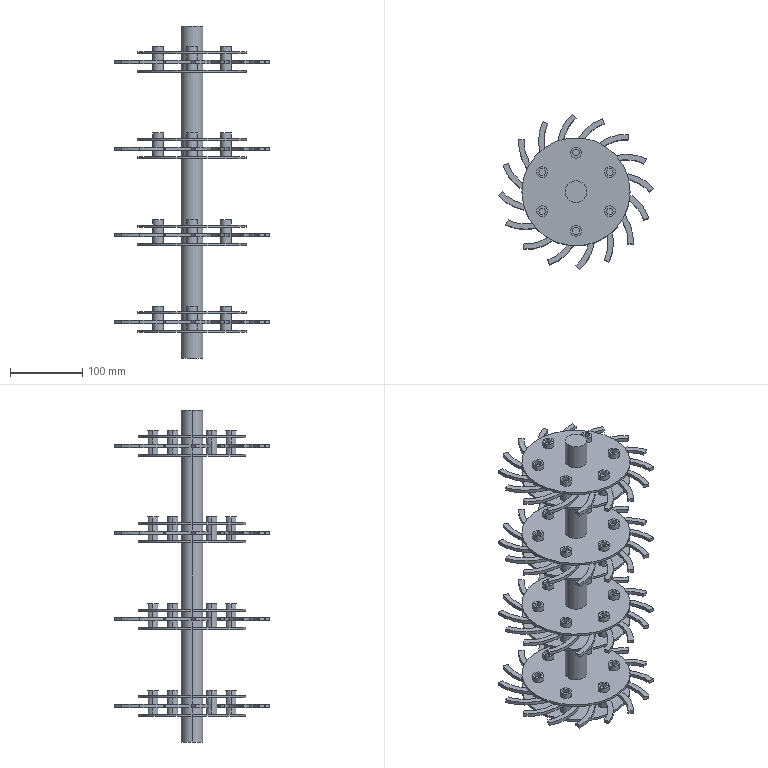Part | SolidWorks | features BaseBody 12, MoveFace 3, ICE 2, Scale 1 | 1 solid | 596 faces | box 214.882 x 214.882 x 460 mm | volume 1059862 mm3 | plane 298 | spline 160 | cylinder 138 | commonest cylinder face diameters 15 x96 30 x26 150 x16